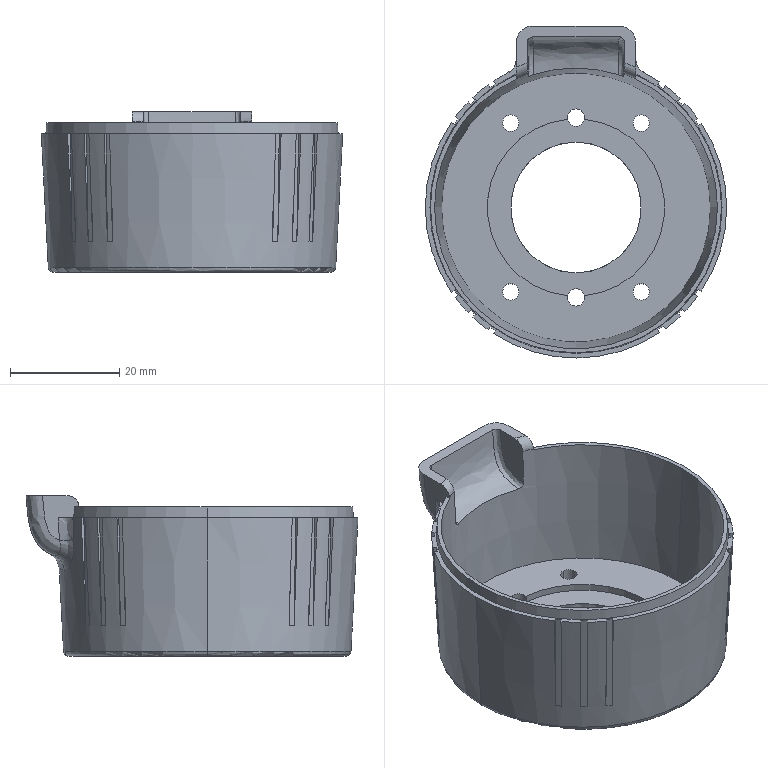Part | NX | features BREP 1 | 1 solid | 111 faces | box 55.272 x 60.87 x 29.488 mm | volume 10698 mm3 | plane 50 | cylinder 23 | cone 23 | spline 11 | torus 4 | commonest cylinder face diameters 3 x8 6 x6 3.2 x4 32.5 x3 24 x2